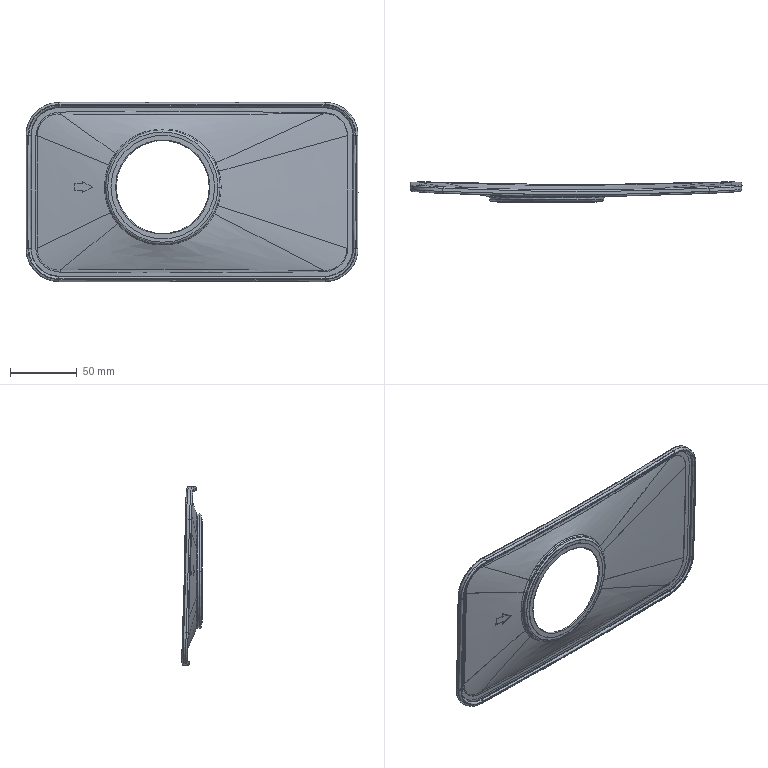Part | STEP file | ZXW722-L-10 | 1 solid | 202 faces | box 249.6 x 15.181 x 134.6 mm | volume 18087 mm3 | spline 149 | plane 33 | cylinder 14 | torus 6 | commonest cylinder face diameters 48.6 x4 49.6 x4 78 x2 85 x2 86 x2